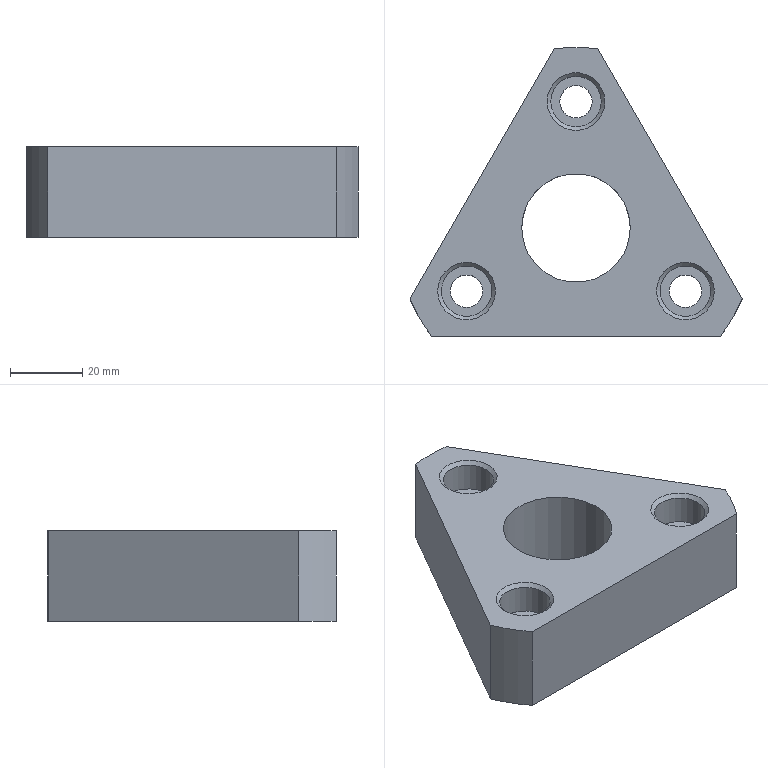NC program | NX | posted with a generic post | part box 91.962 x 80 x 25 mm
Lines 11463 to 11626 of 11626:
(11 , TOOL : D10JING)
N22888 T11 M6
N22890 G54
N22892 G17 G0 G90 X41.096 Y-45.899 S5500 M3
N22894 G43 Z30. H11
N22896 Z-14.
N22898 G94 G1 Z-15. F1000.
N22900 X40.866 Y-45.5
N22902 G3 X40. Y-45. R1.
N22904 G1 X-40.
N22906 G2 X-44. Y-43. R5.
N22908 X-50.579 Y-31.605 R55.
N22910 X-50.311 Y-27.141 R5.
N22912 G1 X-10.311 Y42.141
N22914 G2 X-6.579 Y44.605 R5.
N22916 X6.579 Y44.605 R55.
N22918 X10.311 Y42.141 R5.
N22920 G1 X50.311 Y-27.141
N22922 G2 X50.579 Y-31.605 R5.
N22924 X44. Y-43. R55.
N22926 X40. Y-45. R5.
N22928 G3 X39.134 Y-45.5 R1.
N22930 G1 X38.845 Y-46.
N22932 Z-14.
N22934 G0 X41.096 Y-45.899 Z-24.
N22936 G1 Z-25.
N22938 X40.866 Y-45.5
N22940 G3 X40. Y-45. R1.
N22942 G1 X-40.
N22944 G2 X-44. Y-43. R5.
N22946 X-50.579 Y-31.605 R55.
N22948 X-50.311 Y-27.141 R5.
N22950 G1 X-10.311 Y42.141
N22952 G2 X-6.579 Y44.605 R5.
N22954 X6.579 Y44.605 R55.
N22956 X10.311 Y42.141 R5.
N22958 G1 X50.311 Y-27.141
N22960 G2 X50.579 Y-31.605 R5.
N22962 X44. Y-43. R55.
N22964 X40. Y-45. R5.
N22966 G3 X39.134 Y-45.5 R1.
N22968 G1 X38.845 Y-46.
N22970 Z-24.
N22972 G0 Z30.
N22974 M5
(ZLEVEL_PROFILE_1_COPY_1_COPY , TOOL : D6A45)
N22976 T07 M6
N22978 G54
N22980 G17 G0 G90 X-1.065 Y-22.847 S9500 M3
N22982 G43 Z30. H7
N22984 Z0.
N22986 G94 G1 Z-1. F1000.
N22988 X-0.52 Y-23.791
N22990 G3 X0. Y-24.091 R0.6
N22992 X14.091 Y-10. R14.091
N22994 X0. Y-24.091 R-14.091
N22996 X0.52 Y-23.791 R0.6
N22998 G1 X1.065 Y-22.847
N23000 Z0.
N23002 G0 Z30.
N23004 X40.921 Y-41.952
N23006 Z0.
N23008 G1 Z-1.
N23010 X40.521 Y-41.259
N23012 G3 X40.001 Y-40.959 R0.6
N23014 G1 X-40.001
N23016 G2 X-40.766 Y-40.576 R0.957
N23018 X-46.863 Y-30.017 R50.959
N23020 X-46.811 Y-29.162 R0.957
N23022 G1 X-6.81 Y40.121
N23024 G2 X-6.096 Y40.593 R0.995
N23026 X6.096 Y40.593 R50.959
N23028 X6.81 Y40.121 R0.995
N23030 G1 X46.811 Y-29.162
N23032 G2 X46.863 Y-30.017 R0.957
N23034 X40.766 Y-40.576 R50.959
N23036 X40.001 Y-40.959 R0.957
N23038 G3 X39.481 Y-41.259 R0.6
N23040 G1 X38.962 Y-42.159
N23042 Z0.
N23044 G0 Z30.
(ZLEVEL_PROFILE_1_COPY_1_COPY_COPY , TOOL : D6A45)
N23046 X29.204 Y-32.683
N23048 Z-0.5
N23050 G1 Z-1.5
N23052 X29.791 Y-33.7
N23054 G3 X30.311 Y-34. R0.6
N23056 X36.811 Y-27.5 R6.5
N23058 X30.311 Y-34. R-6.5
N23060 X30.831 Y-33.7 R0.6
N23062 G1 X31.418 Y-32.683
N23064 Z-0.5
N23066 G0 Z30.
N23068 X-31.418
N23070 Z-0.5
N23072 G1 Z-1.5
N23074 X-30.831 Y-33.7
N23076 G3 X-30.311 Y-34. R0.6
N23078 X-23.811 Y-27.5 R6.5
N23080 X-30.311 Y-34. R-6.5
N23082 X-29.791 Y-33.7 R0.6
N23084 G1 X-29.204 Y-32.683
N23086 Z-0.5
N23088 G0 Z30.
N23090 X1.107 Y30.183
N23092 Z-0.5
N23094 G1 Z-1.5
N23096 X0.52 Y31.2
N23098 G3 X0. Y31.5 R0.6
N23100 X-6.5 Y25. R6.5
N23102 X0. Y31.5 R-6.5
N23104 X-0.52 Y31.2 R0.6
N23106 G1 X-1.107 Y30.183
N23108 Z-0.5
N23110 G0 Z30.
N23112 M5
(刀补11 , TOOL : D10JING)
N23114 T11 M6
N23116 G54
N23118 G17 G0 G90 X-8.921 Y-11.524 S5500 M3
N23120 G43 Z30. H11
N23122 Z-14.
N23124 G94 G1 Z-15. F1000.
N23126 X-9.375 Y-12.017
N23128 G3 X-9.594 Y-12.992 R1.
N23130 G1 X-9.592 Y-12.998
N23132 G3 X-7.368 Y-16.835 R10.05
N23134 G1 X-7.357
N23136 X-7.285 Y-16.911
N23138 X-7.287 Y-16.922
N23140 G3 X-7.285 Y-3.077 R-10.05
N23142 G1 Y-3.089
N23144 X-7.367 Y-3.164
N23146 G3 X-9.594 Y-12.992 R10.05
N23148 X-8.859 Y-13.67 R1.
N23150 G1 X-8.206 Y-13.817
N23152 Z-14.
N23154 G0 X-8.921 Y-11.524 Z-24.
N23156 G1 Z-25.
N23158 X-9.375 Y-12.017
N23160 G3 X-9.594 Y-12.992 R1.
N23162 G1 X-9.592 Y-12.998
N23164 G3 X-7.368 Y-16.835 R10.05
N23166 G1 X-7.357
N23168 X-7.284 Y-16.911
N23170 X-7.287 Y-16.922
N23172 G3 X-7.285 Y-3.077 R-10.05
N23174 G1 X-7.284 Y-3.089
N23176 X-7.367 Y-3.164
N23178 G3 X-9.594 Y-12.992 R10.05
N23180 X-8.859 Y-13.67 R1.
N23182 G1 X-8.206 Y-13.817
N23184 Z-24.
N23186 G0 Z30.
N23188 M5
N23190 M2